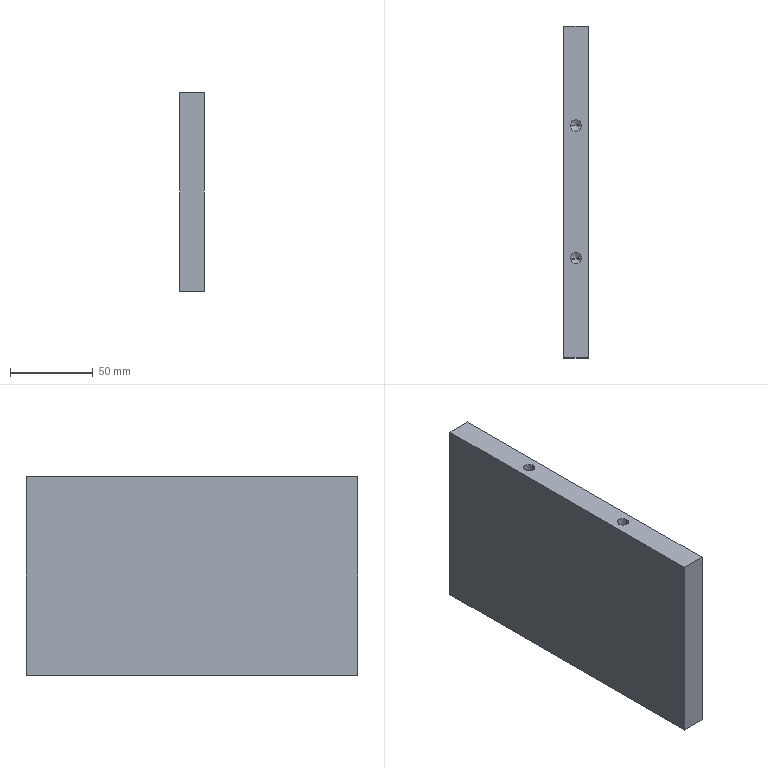Part | STEP file | 11-FGXW-07-0311 | 1 solid | 26 faces | box 15 x 200 x 120 mm | volume 356281 mm3 | cylinder 10 | cone 10 | plane 6 | commonest cylinder face diameters 6.8 x10
STEP:
#1=CARTESIAN_POINT('',(3.4,75.,19.8));
#2=VERTEX_POINT('',#1);
#3=CARTESIAN_POINT('',(-3.4,75.,19.8));
#4=VERTEX_POINT('',#3);
#5=CARTESIAN_POINT('',(0.,75.,19.8));
#6=DIRECTION('',(0.,0.,-1.));
#7=DIRECTION('',(-1.,0.,0.));
#8=AXIS2_PLACEMENT_3D('',#5,#6,#7);
#9=CIRCLE('',#8,3.4);
#10=EDGE_CURVE('',#2,#4,#9,.T.);
#11=ORIENTED_EDGE('',*,*,#10,.F.);
#12=CARTESIAN_POINT('',(3.4,75.,0.));
#13=VERTEX_POINT('',#12);
#14=CARTESIAN_POINT('',(3.4,75.,0.));
#15=DIRECTION('',(0.,0.,-1.));
#16=VECTOR('',#15,1000.);
#17=LINE('',#14,#16);
#18=EDGE_CURVE('',#2,#13,#17,.T.);
#19=ORIENTED_EDGE('',*,*,#18,.T.);
#20=CARTESIAN_POINT('',(-3.4,75.,0.));
#21=VERTEX_POINT('',#20);
#22=CARTESIAN_POINT('',(0.,75.,0.));
#23=DIRECTION('',(0.,0.,-1.));
#24=DIRECTION('',(-1.,0.,0.));
#25=AXIS2_PLACEMENT_3D('',#22,#23,#24);
#26=CIRCLE('',#25,3.4);
#27=EDGE_CURVE('',#13,#21,#26,.T.);
#28=ORIENTED_EDGE('',*,*,#27,.T.);
#29=CARTESIAN_POINT('',(-3.4,75.,0.));
#30=DIRECTION('',(0.,0.,-1.));
#31=VECTOR('',#30,1000.);
#32=LINE('',#29,#31);
#33=EDGE_CURVE('',#4,#21,#32,.T.);
#34=ORIENTED_EDGE('',*,*,#33,.F.);
#35=EDGE_LOOP('',(#11,#19,#28,#34));
#36=FACE_OUTER_BOUND('',#35,.T.);
#37=CARTESIAN_POINT('',(0.,75.,0.));
#38=DIRECTION('',(0.,0.,-1.));
#39=DIRECTION('',(-1.,0.,0.));
#40=AXIS2_PLACEMENT_3D('',#37,#38,#39);
#41=CYLINDRICAL_SURFACE('',#40,3.4);
#42=ADVANCED_FACE('',(#36),#41,.F.);
#43=CARTESIAN_POINT('',(0.,75.,21.843));
#44=VERTEX_POINT('',#43);
#45=CARTESIAN_POINT('',(-3.4,75.,19.8));
#46=DIRECTION('',(-0.8572,0.,-0.515));
#47=VECTOR('',#46,1000.);
#48=LINE('',#45,#47);
#49=EDGE_CURVE('',#44,#4,#48,.T.);
#50=ORIENTED_EDGE('',*,*,#49,.F.);
#51=CARTESIAN_POINT('',(3.4,75.,19.8));
#52=DIRECTION('',(0.8572,0.,-0.515));
#53=VECTOR('',#52,1000.);
#54=LINE('',#51,#53);
#55=EDGE_CURVE('',#44,#2,#54,.T.);
#56=ORIENTED_EDGE('',*,*,#55,.T.);
#57=ORIENTED_EDGE('',*,*,#10,.T.);
#58=EDGE_LOOP('',(#50,#56,#57));
#59=FACE_OUTER_BOUND('',#58,.T.);
#60=CARTESIAN_POINT('',(0.,75.,19.8));
#61=DIRECTION('',(0.,0.,-1.));
#62=DIRECTION('',(-1.,0.,0.));
#63=AXIS2_PLACEMENT_3D('',#60,#61,#62);
#64=CONICAL_SURFACE('',#63,3.4,1.03);
#65=ADVANCED_FACE('',(#59),#64,.F.);
#66=CARTESIAN_POINT('',(3.4,0.,19.8));
#67=VERTEX_POINT('',#66);
#68=CARTESIAN_POINT('',(-3.4,0.,19.8));
#69=VERTEX_POINT('',#68);
#70=CARTESIAN_POINT('',(0.,0.,19.8));
#71=DIRECTION('',(0.,0.,-1.));
#72=DIRECTION('',(-1.,0.,0.));
#73=AXIS2_PLACEMENT_3D('',#70,#71,#72);
#74=CIRCLE('',#73,3.4);
#75=EDGE_CURVE('',#67,#69,#74,.T.);
#76=ORIENTED_EDGE('',*,*,#75,.F.);
#77=CARTESIAN_POINT('',(3.4,0.,0.));
#78=VERTEX_POINT('',#77);
#79=CARTESIAN_POINT('',(3.4,0.,0.));
#80=DIRECTION('',(0.,0.,-1.));
#81=VECTOR('',#80,1000.);
#82=LINE('',#79,#81);
#83=EDGE_CURVE('',#67,#78,#82,.T.);
#84=ORIENTED_EDGE('',*,*,#83,.T.);
#85=CARTESIAN_POINT('',(-3.4,0.,0.));
#86=VERTEX_POINT('',#85);
#87=CARTESIAN_POINT('',(0.,0.,0.));
#88=DIRECTION('',(0.,0.,-1.));
#89=DIRECTION('',(-1.,0.,0.));
#90=AXIS2_PLACEMENT_3D('',#87,#88,#89);
#91=CIRCLE('',#90,3.4);
#92=EDGE_CURVE('',#78,#86,#91,.T.);
#93=ORIENTED_EDGE('',*,*,#92,.T.);
#94=CARTESIAN_POINT('',(-3.4,0.,0.));
#95=DIRECTION('',(0.,0.,-1.));
#96=VECTOR('',#95,1000.);
#97=LINE('',#94,#96);
#98=EDGE_CURVE('',#69,#86,#97,.T.);
#99=ORIENTED_EDGE('',*,*,#98,.F.);
#100=EDGE_LOOP('',(#76,#84,#93,#99));
#101=FACE_OUTER_BOUND('',#100,.T.);
#102=CARTESIAN_POINT('',(0.,0.,0.));
#103=DIRECTION('',(0.,0.,-1.));
#104=DIRECTION('',(-1.,0.,0.));
#105=AXIS2_PLACEMENT_3D('',#102,#103,#104);
#106=CYLINDRICAL_SURFACE('',#105,3.4);
#107=ADVANCED_FACE('',(#101),#106,.F.);
#108=CARTESIAN_POINT('',(0.,0.,21.843));
#109=VERTEX_POINT('',#108);
#110=CARTESIAN_POINT('',(-3.4,0.,19.8));
#111=DIRECTION('',(-0.8572,0.,-0.515));
#112=VECTOR('',#111,1000.);
#113=LINE('',#110,#112);
#114=EDGE_CURVE('',#109,#69,#113,.T.);
#115=ORIENTED_EDGE('',*,*,#114,.F.);
#116=CARTESIAN_POINT('',(3.4,0.,19.8));
#117=DIRECTION('',(0.8572,0.,-0.515));
#118=VECTOR('',#117,1000.);
#119=LINE('',#116,#118);
#120=EDGE_CURVE('',#109,#67,#119,.T.);
#121=ORIENTED_EDGE('',*,*,#120,.T.);
#122=ORIENTED_EDGE('',*,*,#75,.T.);
#123=EDGE_LOOP('',(#115,#121,#122));
#124=FACE_OUTER_BOUND('',#123,.T.);
#125=CARTESIAN_POINT('',(0.,0.,19.8));
#126=DIRECTION('',(0.,0.,-1.));
#127=DIRECTION('',(-1.,0.,0.));
#128=AXIS2_PLACEMENT_3D('',#125,#126,#127);
#129=CONICAL_SURFACE('',#128,3.4,1.03);
#130=ADVANCED_FACE('',(#124),#129,.F.);
#131=CARTESIAN_POINT('',(3.4,-75.,19.8));
#132=VERTEX_POINT('',#131);
#133=CARTESIAN_POINT('',(-3.4,-75.,19.8));
#134=VERTEX_POINT('',#133);
#135=CARTESIAN_POINT('',(0.,-75.,19.8));
#136=DIRECTION('',(0.,0.,-1.));
#137=DIRECTION('',(-1.,0.,0.));
#138=AXIS2_PLACEMENT_3D('',#135,#136,#137);
#139=CIRCLE('',#138,3.4);
#140=EDGE_CURVE('',#132,#134,#139,.T.);
#141=ORIENTED_EDGE('',*,*,#140,.F.);
#142=CARTESIAN_POINT('',(3.4,-75.,0.));
#143=VERTEX_POINT('',#142);
#144=CARTESIAN_POINT('',(3.4,-75.,0.));
#145=DIRECTION('',(0.,0.,-1.));
#146=VECTOR('',#145,1000.);
#147=LINE('',#144,#146);
#148=EDGE_CURVE('',#132,#143,#147,.T.);
#149=ORIENTED_EDGE('',*,*,#148,.T.);
#150=CARTESIAN_POINT('',(-3.4,-75.,0.));
#151=VERTEX_POINT('',#150);
#152=CARTESIAN_POINT('',(0.,-75.,0.));
#153=DIRECTION('',(0.,0.,-1.));
#154=DIRECTION('',(-1.,0.,0.));
#155=AXIS2_PLACEMENT_3D('',#152,#153,#154);
#156=CIRCLE('',#155,3.4);
#157=EDGE_CURVE('',#143,#151,#156,.T.);
#158=ORIENTED_EDGE('',*,*,#157,.T.);
#159=CARTESIAN_POINT('',(-3.4,-75.,0.));
#160=DIRECTION('',(0.,0.,-1.));
#161=VECTOR('',#160,1000.);
#162=LINE('',#159,#161);
#163=EDGE_CURVE('',#134,#151,#162,.T.);
#164=ORIENTED_EDGE('',*,*,#163,.F.);
#165=EDGE_LOOP('',(#141,#149,#158,#164));
#166=FACE_OUTER_BOUND('',#165,.T.);
#167=CARTESIAN_POINT('',(0.,-75.,0.));
#168=DIRECTION('',(0.,0.,-1.));
#169=DIRECTION('',(-1.,0.,0.));
#170=AXIS2_PLACEMENT_3D('',#167,#168,#169);
#171=CYLINDRICAL_SURFACE('',#170,3.4);
#172=ADVANCED_FACE('',(#166),#171,.F.);
#173=CARTESIAN_POINT('',(0.,-75.,21.843));
#174=VERTEX_POINT('',#173);
#175=CARTESIAN_POINT('',(-3.4,-75.,19.8));
#176=DIRECTION('',(-0.8572,0.,-0.515));
#177=VECTOR('',#176,1000.);
#178=LINE('',#175,#177);
#179=EDGE_CURVE('',#174,#134,#178,.T.);
#180=ORIENTED_EDGE('',*,*,#179,.F.);
#181=CARTESIAN_POINT('',(3.4,-75.,19.8));
#182=DIRECTION('',(0.8572,0.,-0.515));
#183=VECTOR('',#182,1000.);
#184=LINE('',#181,#183);
#185=EDGE_CURVE('',#174,#132,#184,.T.);
#186=ORIENTED_EDGE('',*,*,#185,.T.);
#187=ORIENTED_EDGE('',*,*,#140,.T.);
#188=EDGE_LOOP('',(#180,#186,#187));
#189=FACE_OUTER_BOUND('',#188,.T.);
#190=CARTESIAN_POINT('',(0.,-75.,19.8));
#191=DIRECTION('',(0.,0.,-1.));
#192=DIRECTION('',(-1.,0.,0.));
#193=AXIS2_PLACEMENT_3D('',#190,#191,#192);
#194=CONICAL_SURFACE('',#193,3.4,1.03);
#195=ADVANCED_FACE('',(#189),#194,.F.);
#196=CARTESIAN_POINT('',(-3.4,-40.,100.2));
#197=VERTEX_POINT('',#196);
#198=CARTESIAN_POINT('',(3.4,-40.,100.2));
#199=VERTEX_POINT('',#198);
#200=CARTESIAN_POINT('',(0.,-40.,100.2));
#201=DIRECTION('',(0.,0.,1.));
#202=DIRECTION('',(1.,0.,0.));
#203=AXIS2_PLACEMENT_3D('',#200,#201,#202);
#204=CIRCLE('',#203,3.4);
#205=EDGE_CURVE('',#197,#199,#204,.T.);
#206=ORIENTED_EDGE('',*,*,#205,.F.);
#207=CARTESIAN_POINT('',(-3.4,-40.,120.));
#208=VERTEX_POINT('',#207);
#209=CARTESIAN_POINT('',(-3.4,-40.,120.));
#210=DIRECTION('',(0.,0.,1.));
#211=VECTOR('',#210,1000.);
#212=LINE('',#209,#211);
#213=EDGE_CURVE('',#197,#208,#212,.T.);
#214=ORIENTED_EDGE('',*,*,#213,.T.);
#215=CARTESIAN_POINT('',(3.4,-40.,120.));
#216=VERTEX_POINT('',#215);
#217=CARTESIAN_POINT('',(0.,-40.,120.));
#218=DIRECTION('',(0.,0.,1.));
#219=DIRECTION('',(1.,0.,0.));
#220=AXIS2_PLACEMENT_3D('',#217,#218,#219);
#221=CIRCLE('',#220,3.4);
#222=EDGE_CURVE('',#208,#216,#221,.T.);
#223=ORIENTED_EDGE('',*,*,#222,.T.);
#224=CARTESIAN_POINT('',(3.4,-40.,120.));
#225=DIRECTION('',(0.,0.,1.));
#226=VECTOR('',#225,1000.);
#227=LINE('',#224,#226);
#228=EDGE_CURVE('',#199,#216,#227,.T.);
#229=ORIENTED_EDGE('',*,*,#228,.F.);
#230=EDGE_LOOP('',(#206,#214,#223,#229));
#231=FACE_OUTER_BOUND('',#230,.T.);
#232=CARTESIAN_POINT('',(0.,-40.,120.));
#233=DIRECTION('',(0.,0.,1.));
#234=DIRECTION('',(1.,0.,0.));
#235=AXIS2_PLACEMENT_3D('',#232,#233,#234);
#236=CYLINDRICAL_SURFACE('',#235,3.4);
#237=ADVANCED_FACE('',(#231),#236,.F.);
#238=CARTESIAN_POINT('',(0.,-40.,98.157));
#239=VERTEX_POINT('',#238);
#240=CARTESIAN_POINT('',(3.4,-40.,100.2));
#241=DIRECTION('',(0.8572,0.,0.515));
#242=VECTOR('',#241,1000.);
#243=LINE('',#240,#242);
#244=EDGE_CURVE('',#239,#199,#243,.T.);
#245=ORIENTED_EDGE('',*,*,#244,.F.);
#246=CARTESIAN_POINT('',(-3.4,-40.,100.2));
#247=DIRECTION('',(-0.8572,0.,0.515));
#248=VECTOR('',#247,1000.);
#249=LINE('',#246,#248);
#250=EDGE_CURVE('',#239,#197,#249,.T.);
#251=ORIENTED_EDGE('',*,*,#250,.T.);
#252=ORIENTED_EDGE('',*,*,#205,.T.);
#253=EDGE_LOOP('',(#245,#251,#252));
#254=FACE_OUTER_BOUND('',#253,.T.);
#255=CARTESIAN_POINT('',(0.,-40.,100.2));
#256=DIRECTION('',(0.,0.,1.));
#257=DIRECTION('',(1.,0.,0.));
#258=AXIS2_PLACEMENT_3D('',#255,#256,#257);
#259=CONICAL_SURFACE('',#258,3.4,1.03);
#260=ADVANCED_FACE('',(#254),#259,.F.);
#261=CARTESIAN_POINT('',(-3.4,40.,100.2));
#262=VERTEX_POINT('',#261);
#263=CARTESIAN_POINT('',(3.4,40.,100.2));
#264=VERTEX_POINT('',#263);
#265=CARTESIAN_POINT('',(0.,40.,100.2));
#266=DIRECTION('',(0.,0.,1.));
#267=DIRECTION('',(1.,0.,0.));
#268=AXIS2_PLACEMENT_3D('',#265,#266,#267);
#269=CIRCLE('',#268,3.4);
#270=EDGE_CURVE('',#262,#264,#269,.T.);
#271=ORIENTED_EDGE('',*,*,#270,.F.);
#272=CARTESIAN_POINT('',(-3.4,40.,120.));
#273=VERTEX_POINT('',#272);
#274=CARTESIAN_POINT('',(-3.4,40.,120.));
#275=DIRECTION('',(0.,0.,1.));
#276=VECTOR('',#275,1000.);
#277=LINE('',#274,#276);
#278=EDGE_CURVE('',#262,#273,#277,.T.);
#279=ORIENTED_EDGE('',*,*,#278,.T.);
#280=CARTESIAN_POINT('',(3.4,40.,120.));
#281=VERTEX_POINT('',#280);
#282=CARTESIAN_POINT('',(0.,40.,120.));
#283=DIRECTION('',(0.,0.,1.));
#284=DIRECTION('',(1.,0.,0.));
#285=AXIS2_PLACEMENT_3D('',#282,#283,#284);
#286=CIRCLE('',#285,3.4);
#287=EDGE_CURVE('',#273,#281,#286,.T.);
#288=ORIENTED_EDGE('',*,*,#287,.T.);
#289=CARTESIAN_POINT('',(3.4,40.,120.));
#290=DIRECTION('',(0.,0.,1.));
#291=VECTOR('',#290,1000.);
#292=LINE('',#289,#291);
#293=EDGE_CURVE('',#264,#281,#292,.T.);
#294=ORIENTED_EDGE('',*,*,#293,.F.);
#295=EDGE_LOOP('',(#271,#279,#288,#294));
#296=FACE_OUTER_BOUND('',#295,.T.);
#297=CARTESIAN_POINT('',(0.,40.,120.));
#298=DIRECTION('',(0.,0.,1.));
#299=DIRECTION('',(1.,0.,0.));
#300=AXIS2_PLACEMENT_3D('',#297,#298,#299);
#301=CYLINDRICAL_SURFACE('',#300,3.4);
#302=ADVANCED_FACE('',(#296),#301,.F.);
#303=CARTESIAN_POINT('',(0.,40.,98.157));
#304=VERTEX_POINT('',#303);
#305=CARTESIAN_POINT('',(3.4,40.,100.2));
#306=DIRECTION('',(0.8572,0.,0.515));
#307=VECTOR('',#306,1000.);
#308=LINE('',#305,#307);
#309=EDGE_CURVE('',#304,#264,#308,.T.);
#310=ORIENTED_EDGE('',*,*,#309,.F.);
#311=CARTESIAN_POINT('',(-3.4,40.,100.2));
#312=DIRECTION('',(-0.8572,0.,0.515));
#313=VECTOR('',#312,1000.);
#314=LINE('',#311,#313);
#315=EDGE_CURVE('',#304,#262,#314,.T.);
#316=ORIENTED_EDGE('',*,*,#315,.T.);
#317=ORIENTED_EDGE('',*,*,#270,.T.);
#318=EDGE_LOOP('',(#310,#316,#317));
#319=FACE_OUTER_BOUND('',#318,.T.);
#320=CARTESIAN_POINT('',(0.,40.,100.2));
#321=DIRECTION('',(0.,0.,1.));
#322=DIRECTION('',(1.,0.,0.));
#323=AXIS2_PLACEMENT_3D('',#320,#321,#322);
#324=CONICAL_SURFACE('',#323,3.4,1.03);
#325=ADVANCED_FACE('',(#319),#324,.F.);
#326=CARTESIAN_POINT('',(7.5,-100.,0.));
#327=VERTEX_POINT('',#326);
#328=CARTESIAN_POINT('',(7.5,100.,0.));
#329=VERTEX_POINT('',#328);
#330=CARTESIAN_POINT('',(7.5,-100.,0.));
#331=DIRECTION('',(0.,1.,0.));
#332=VECTOR('',#331,1000.);
#333=LINE('',#330,#332);
#334=EDGE_CURVE('',#327,#329,#333,.T.);
#335=ORIENTED_EDGE('',*,*,#334,.T.);
#336=CARTESIAN_POINT('',(7.5,100.,120.));
#337=VERTEX_POINT('',#336);
#338=CARTESIAN_POINT('',(7.5,100.,120.));
#339=DIRECTION('',(0.,0.,-1.));
#340=VECTOR('',#339,1000.);
#341=LINE('',#338,#340);
#342=EDGE_CURVE('',#337,#329,#341,.T.);
#343=ORIENTED_EDGE('',*,*,#342,.F.);
#344=CARTESIAN_POINT('',(7.5,-100.,120.));
#345=VERTEX_POINT('',#344);
#346=CARTESIAN_POINT('',(7.5,-100.,120.));
#347=DIRECTION('',(0.,1.,0.));
#348=VECTOR('',#347,1000.);
#349=LINE('',#346,#348);
#350=EDGE_CURVE('',#345,#337,#349,.T.);
#351=ORIENTED_EDGE('',*,*,#350,.F.);
#352=CARTESIAN_POINT('',(7.5,-100.,120.));
#353=DIRECTION('',(0.,0.,-1.));
#354=VECTOR('',#353,1000.);
#355=LINE('',#352,#354);
#356=EDGE_CURVE('',#345,#327,#355,.T.);
#357=ORIENTED_EDGE('',*,*,#356,.T.);
#358=EDGE_LOOP('',(#335,#343,#351,#357));
#359=FACE_OUTER_BOUND('',#358,.T.);
#360=CARTESIAN_POINT('',(7.5,-100.,120.));
#361=DIRECTION('',(-1.,0.,0.));
#362=DIRECTION('',(0.,0.,1.));
#363=AXIS2_PLACEMENT_3D('',#360,#361,#362);
#364=PLANE('',#363);
#365=ADVANCED_FACE('',(#359),#364,.F.);
#366=CARTESIAN_POINT('',(-7.5,100.,0.));
#367=VERTEX_POINT('',#366);
#368=CARTESIAN_POINT('',(-7.5,100.,0.));
#369=DIRECTION('',(-1.,0.,0.));
#370=VECTOR('',#369,1000.);
#371=LINE('',#368,#370);
#372=EDGE_CURVE('',#329,#367,#371,.T.);
#373=ORIENTED_EDGE('',*,*,#372,.T.);
#374=CARTESIAN_POINT('',(-7.5,100.,120.));
#375=VERTEX_POINT('',#374);
#376=CARTESIAN_POINT('',(-7.5,100.,120.));
#377=DIRECTION('',(0.,0.,-1.));
#378=VECTOR('',#377,1000.);
#379=LINE('',#376,#378);
#380=EDGE_CURVE('',#375,#367,#379,.T.);
#381=ORIENTED_EDGE('',*,*,#380,.F.);
#382=CARTESIAN_POINT('',(-7.5,100.,120.));
#383=DIRECTION('',(-1.,0.,0.));
#384=VECTOR('',#383,1000.);
#385=LINE('',#382,#384);
#386=EDGE_CURVE('',#337,#375,#385,.T.);
#387=ORIENTED_EDGE('',*,*,#386,.F.);
#388=ORIENTED_EDGE('',*,*,#342,.T.);
#389=EDGE_LOOP('',(#373,#381,#387,#388));
#390=FACE_OUTER_BOUND('',#389,.T.);
#391=CARTESIAN_POINT('',(-7.5,100.,120.));
#392=DIRECTION('',(0.,-1.,0.));
#393=DIRECTION('',(0.,0.,-1.));
#394=AXIS2_PLACEMENT_3D('',#391,#392,#393);
#395=PLANE('',#394);
#396=ADVANCED_FACE('',(#390),#395,.F.);
#397=CARTESIAN_POINT('',(-7.5,-100.,0.));
#398=VERTEX_POINT('',#397);
#399=CARTESIAN_POINT('',(-7.5,-100.,0.));
#400=DIRECTION('',(0.,-1.,0.));
#401=VECTOR('',#400,1000.);
#402=LINE('',#399,#401);
#403=EDGE_CURVE('',#367,#398,#402,.T.);
#404=ORIENTED_EDGE('',*,*,#403,.T.);
#405=CARTESIAN_POINT('',(-7.5,-100.,120.));
#406=VERTEX_POINT('',#405);
#407=CARTESIAN_POINT('',(-7.5,-100.,120.));
#408=DIRECTION('',(0.,0.,-1.));
#409=VECTOR('',#408,1000.);
#410=LINE('',#407,#409);
#411=EDGE_CURVE('',#406,#398,#410,.T.);
#412=ORIENTED_EDGE('',*,*,#411,.F.);
#413=CARTESIAN_POINT('',(-7.5,-100.,120.));
#414=DIRECTION('',(0.,-1.,0.));
#415=VECTOR('',#414,1000.);
#416=LINE('',#413,#415);
#417=EDGE_CURVE('',#375,#406,#416,.T.);
#418=ORIENTED_EDGE('',*,*,#417,.F.);
#419=ORIENTED_EDGE('',*,*,#380,.T.);
#420=EDGE_LOOP('',(#404,#412,#418,#419));
#421=FACE_OUTER_BOUND('',#420,.T.);
#422=CARTESIAN_POINT('',(-7.5,-100.,120.));
#423=DIRECTION('',(1.,0.,0.));
#424=DIRECTION('',(0.,0.,-1.));
#425=AXIS2_PLACEMENT_3D('',#422,#423,#424);
#426=PLANE('',#425);
#427=ADVANCED_FACE('',(#421),#426,.F.);
#428=CARTESIAN_POINT('',(-7.5,-100.,0.));
#429=DIRECTION('',(1.,0.,0.));
#430=VECTOR('',#429,1000.);
#431=LINE('',#428,#430);
#432=EDGE_CURVE('',#398,#327,#431,.T.);
#433=ORIENTED_EDGE('',*,*,#432,.T.);
#434=ORIENTED_EDGE('',*,*,#356,.F.);
#435=CARTESIAN_POINT('',(-7.5,-100.,120.));
#436=DIRECTION('',(1.,0.,0.));
#437=VECTOR('',#436,1000.);
#438=LINE('',#435,#437);
#439=EDGE_CURVE('',#406,#345,#438,.T.);
#440=ORIENTED_EDGE('',*,*,#439,.F.);
#441=ORIENTED_EDGE('',*,*,#411,.T.);
#442=EDGE_LOOP('',(#433,#434,#440,#441));
#443=FACE_OUTER_BOUND('',#442,.T.);
#444=CARTESIAN_POINT('',(-7.5,-100.,120.));
#445=DIRECTION('',(0.,1.,0.));
#446=DIRECTION('',(0.,0.,1.));
#447=AXIS2_PLACEMENT_3D('',#444,#445,#446);
#448=PLANE('',#447);
#449=ADVANCED_FACE('',(#443),#448,.F.);
#450=CARTESIAN_POINT('',(0.,-40.,120.));
#451=DIRECTION('',(0.,0.,1.));
#452=DIRECTION('',(1.,0.,0.));
#453=AXIS2_PLACEMENT_3D('',#450,#451,#452);
#454=CIRCLE('',#453,3.4);
#455=EDGE_CURVE('',#216,#208,#454,.T.);
#456=ORIENTED_EDGE('',*,*,#455,.F.);
#457=ORIENTED_EDGE('',*,*,#222,.F.);
#458=EDGE_LOOP('',(#456,#457));
#459=FACE_BOUND('',#458,.T.);
#460=CARTESIAN_POINT('',(0.,40.,120.));
#461=DIRECTION('',(0.,0.,1.));
#462=DIRECTION('',(1.,0.,0.));
#463=AXIS2_PLACEMENT_3D('',#460,#461,#462);
#464=CIRCLE('',#463,3.4);
#465=EDGE_CURVE('',#281,#273,#464,.T.);
#466=ORIENTED_EDGE('',*,*,#465,.F.);
#467=ORIENTED_EDGE('',*,*,#287,.F.);
#468=EDGE_LOOP('',(#466,#467));
#469=FACE_BOUND('',#468,.T.);
#470=ORIENTED_EDGE('',*,*,#350,.T.);
#471=ORIENTED_EDGE('',*,*,#386,.T.);
#472=ORIENTED_EDGE('',*,*,#417,.T.);
#473=ORIENTED_EDGE('',*,*,#439,.T.);
#474=EDGE_LOOP('',(#470,#471,#472,#473));
#475=FACE_OUTER_BOUND('',#474,.T.);
#476=CARTESIAN_POINT('',(0.,0.,120.));
#477=DIRECTION('',(0.,0.,-1.));
#478=DIRECTION('',(-1.,0.,0.));
#479=AXIS2_PLACEMENT_3D('',#476,#477,#478);
#480=PLANE('',#479);
#481=ADVANCED_FACE('',(#459,#469,#475),#480,.F.);
#482=CARTESIAN_POINT('',(0.,75.,0.));
#483=DIRECTION('',(0.,0.,-1.));
#484=DIRECTION('',(-1.,0.,0.));
#485=AXIS2_PLACEMENT_3D('',#482,#483,#484);
#486=CIRCLE('',#485,3.4);
#487=EDGE_CURVE('',#21,#13,#486,.T.);
#488=ORIENTED_EDGE('',*,*,#487,.F.);
#489=ORIENTED_EDGE('',*,*,#27,.F.);
#490=EDGE_LOOP('',(#488,#489));
#491=FACE_BOUND('',#490,.T.);
#492=CARTESIAN_POINT('',(0.,0.,0.));
#493=DIRECTION('',(0.,0.,-1.));
#494=DIRECTION('',(-1.,0.,0.));
#495=AXIS2_PLACEMENT_3D('',#492,#493,#494);
#496=CIRCLE('',#495,3.4);
#497=EDGE_CURVE('',#86,#78,#496,.T.);
#498=ORIENTED_EDGE('',*,*,#497,.F.);
#499=ORIENTED_EDGE('',*,*,#92,.F.);
#500=EDGE_LOOP('',(#498,#499));
#501=FACE_BOUND('',#500,.T.);
#502=CARTESIAN_POINT('',(0.,-75.,0.));
#503=DIRECTION('',(0.,0.,-1.));
#504=DIRECTION('',(-1.,0.,0.));
#505=AXIS2_PLACEMENT_3D('',#502,#503,#504);
#506=CIRCLE('',#505,3.4);
#507=EDGE_CURVE('',#151,#143,#506,.T.);
#508=ORIENTED_EDGE('',*,*,#507,.F.);
#509=ORIENTED_EDGE('',*,*,#157,.F.);
#510=EDGE_LOOP('',(#508,#509));
#511=FACE_BOUND('',#510,.T.);
#512=ORIENTED_EDGE('',*,*,#334,.F.);
#513=ORIENTED_EDGE('',*,*,#432,.F.);
#514=ORIENTED_EDGE('',*,*,#403,.F.);
#515=ORIENTED_EDGE('',*,*,#372,.F.);
#516=EDGE_LOOP('',(#512,#513,#514,#515));
#517=FACE_OUTER_BOUND('',#516,.T.);
#518=CARTESIAN_POINT('',(0.,0.,0.));
#519=DIRECTION('',(0.,0.,-1.));
#520=DIRECTION('',(-1.,0.,0.));
#521=AXIS2_PLACEMENT_3D('',#518,#519,#520);
#522=PLANE('',#521);
#523=ADVANCED_FACE('',(#491,#501,#511,#517),#522,.T.);
#524=ORIENTED_EDGE('',*,*,#315,.F.);
#525=ORIENTED_EDGE('',*,*,#309,.T.);
#526=CARTESIAN_POINT('',(0.,40.,100.2));
#527=DIRECTION('',(0.,0.,1.));
#528=DIRECTION('',(1.,0.,0.));
#529=AXIS2_PLACEMENT_3D('',#526,#527,#528);
#530=CIRCLE('',#529,3.4);
#531=EDGE_CURVE('',#264,#262,#530,.T.);
#532=ORIENTED_EDGE('',*,*,#531,.T.);
#533=EDGE_LOOP('',(#524,#525,#532));
#534=FACE_OUTER_BOUND('',#533,.T.);
#535=CARTESIAN_POINT('',(0.,40.,100.2));
#536=DIRECTION('',(0.,0.,1.));
#537=DIRECTION('',(1.,0.,0.));
#538=AXIS2_PLACEMENT_3D('',#535,#536,#537);
#539=CONICAL_SURFACE('',#538,3.4,1.03);
#540=ADVANCED_FACE('',(#534),#539,.F.);
#541=ORIENTED_EDGE('',*,*,#278,.F.);
#542=ORIENTED_EDGE('',*,*,#531,.F.);
#543=ORIENTED_EDGE('',*,*,#293,.T.);
#544=ORIENTED_EDGE('',*,*,#465,.T.);
#545=EDGE_LOOP('',(#541,#542,#543,#544));
#546=FACE_OUTER_BOUND('',#545,.T.);
#547=CARTESIAN_POINT('',(0.,40.,120.));
#548=DIRECTION('',(0.,0.,1.));
#549=DIRECTION('',(1.,0.,0.));
#550=AXIS2_PLACEMENT_3D('',#547,#548,#549);
#551=CYLINDRICAL_SURFACE('',#550,3.4);
#552=ADVANCED_FACE('',(#546),#551,.F.);
#553=ORIENTED_EDGE('',*,*,#250,.F.);
#554=ORIENTED_EDGE('',*,*,#244,.T.);
#555=CARTESIAN_POINT('',(0.,-40.,100.2));
#556=DIRECTION('',(0.,0.,1.));
#557=DIRECTION('',(1.,0.,0.));
#558=AXIS2_PLACEMENT_3D('',#555,#556,#557);
#559=CIRCLE('',#558,3.4);
#560=EDGE_CURVE('',#199,#197,#559,.T.);
#561=ORIENTED_EDGE('',*,*,#560,.T.);
#562=EDGE_LOOP('',(#553,#554,#561));
#563=FACE_OUTER_BOUND('',#562,.T.);
#564=CARTESIAN_POINT('',(0.,-40.,100.2));
#565=DIRECTION('',(0.,0.,1.));
#566=DIRECTION('',(1.,0.,0.));
#567=AXIS2_PLACEMENT_3D('',#564,#565,#566);
#568=CONICAL_SURFACE('',#567,3.4,1.03);
#569=ADVANCED_FACE('',(#563),#568,.F.);
#570=ORIENTED_EDGE('',*,*,#213,.F.);
#571=ORIENTED_EDGE('',*,*,#560,.F.);
#572=ORIENTED_EDGE('',*,*,#228,.T.);
#573=ORIENTED_EDGE('',*,*,#455,.T.);
#574=EDGE_LOOP('',(#570,#571,#572,#573));
#575=FACE_OUTER_BOUND('',#574,.T.);
#576=CARTESIAN_POINT('',(0.,-40.,120.));
#577=DIRECTION('',(0.,0.,1.));
#578=DIRECTION('',(1.,0.,0.));
#579=AXIS2_PLACEMENT_3D('',#576,#577,#578);
#580=CYLINDRICAL_SURFACE('',#579,3.4);
#581=ADVANCED_FACE('',(#575),#580,.F.);
#582=ORIENTED_EDGE('',*,*,#185,.F.);
#583=ORIENTED_EDGE('',*,*,#179,.T.);
#584=CARTESIAN_POINT('',(0.,-75.,19.8));
#585=DIRECTION('',(0.,0.,-1.));
#586=DIRECTION('',(-1.,0.,0.));
#587=AXIS2_PLACEMENT_3D('',#584,#585,#586);
#588=CIRCLE('',#587,3.4);
#589=EDGE_CURVE('',#134,#132,#588,.T.);
#590=ORIENTED_EDGE('',*,*,#589,.T.);
#591=EDGE_LOOP('',(#582,#583,#590));
#592=FACE_OUTER_BOUND('',#591,.T.);
#593=CARTESIAN_POINT('',(0.,-75.,19.8));
#594=DIRECTION('',(0.,0.,-1.));
#595=DIRECTION('',(-1.,0.,0.));
#596=AXIS2_PLACEMENT_3D('',#593,#594,#595);
#597=CONICAL_SURFACE('',#596,3.4,1.03);
#598=ADVANCED_FACE('',(#592),#597,.F.);
#599=ORIENTED_EDGE('',*,*,#148,.F.);
#600=ORIENTED_EDGE('',*,*,#589,.F.);
#601=ORIENTED_EDGE('',*,*,#163,.T.);
#602=ORIENTED_EDGE('',*,*,#507,.T.);
#603=EDGE_LOOP('',(#599,#600,#601,#602));
#604=FACE_OUTER_BOUND('',#603,.T.);
#605=CARTESIAN_POINT('',(0.,-75.,0.));
#606=DIRECTION('',(0.,0.,-1.));
#607=DIRECTION('',(-1.,0.,0.));
#608=AXIS2_PLACEMENT_3D('',#605,#606,#607);
#609=CYLINDRICAL_SURFACE('',#608,3.4);
#610=ADVANCED_FACE('',(#604),#609,.F.);
#611=ORIENTED_EDGE('',*,*,#120,.F.);
#612=ORIENTED_EDGE('',*,*,#114,.T.);
#613=CARTESIAN_POINT('',(0.,0.,19.8));
#614=DIRECTION('',(0.,0.,-1.));
#615=DIRECTION('',(-1.,0.,0.));
#616=AXIS2_PLACEMENT_3D('',#613,#614,#615);
#617=CIRCLE('',#616,3.4);
#618=EDGE_CURVE('',#69,#67,#617,.T.);
#619=ORIENTED_EDGE('',*,*,#618,.T.);
#620=EDGE_LOOP('',(#611,#612,#619));
#621=FACE_OUTER_BOUND('',#620,.T.);
#622=CARTESIAN_POINT('',(0.,0.,19.8));
#623=DIRECTION('',(0.,0.,-1.));
#624=DIRECTION('',(-1.,0.,0.));
#625=AXIS2_PLACEMENT_3D('',#622,#623,#624);
#626=CONICAL_SURFACE('',#625,3.4,1.03);
#627=ADVANCED_FACE('',(#621),#626,.F.);
#628=ORIENTED_EDGE('',*,*,#83,.F.);
#629=ORIENTED_EDGE('',*,*,#618,.F.);
#630=ORIENTED_EDGE('',*,*,#98,.T.);
#631=ORIENTED_EDGE('',*,*,#497,.T.);
#632=EDGE_LOOP('',(#628,#629,#630,#631));
#633=FACE_OUTER_BOUND('',#632,.T.);
#634=CARTESIAN_POINT('',(0.,0.,0.));
#635=DIRECTION('',(0.,0.,-1.));
#636=DIRECTION('',(-1.,0.,0.));
#637=AXIS2_PLACEMENT_3D('',#634,#635,#636);
#638=CYLINDRICAL_SURFACE('',#637,3.4);
#639=ADVANCED_FACE('',(#633),#638,.F.);
#640=ORIENTED_EDGE('',*,*,#55,.F.);
#641=ORIENTED_EDGE('',*,*,#49,.T.);
#642=CARTESIAN_POINT('',(0.,75.,19.8));
#643=DIRECTION('',(0.,0.,-1.));
#644=DIRECTION('',(-1.,0.,0.));
#645=AXIS2_PLACEMENT_3D('',#642,#643,#644);
#646=CIRCLE('',#645,3.4);
#647=EDGE_CURVE('',#4,#2,#646,.T.);
#648=ORIENTED_EDGE('',*,*,#647,.T.);
#649=EDGE_LOOP('',(#640,#641,#648));
#650=FACE_OUTER_BOUND('',#649,.T.);
#651=CARTESIAN_POINT('',(0.,75.,19.8));
#652=DIRECTION('',(0.,0.,-1.));
#653=DIRECTION('',(-1.,0.,0.));
#654=AXIS2_PLACEMENT_3D('',#651,#652,#653);
#655=CONICAL_SURFACE('',#654,3.4,1.03);
#656=ADVANCED_FACE('',(#650),#655,.F.);
#657=ORIENTED_EDGE('',*,*,#18,.F.);
#658=ORIENTED_EDGE('',*,*,#647,.F.);
#659=ORIENTED_EDGE('',*,*,#33,.T.);
#660=ORIENTED_EDGE('',*,*,#487,.T.);
#661=EDGE_LOOP('',(#657,#658,#659,#660));
#662=FACE_OUTER_BOUND('',#661,.T.);
#663=CARTESIAN_POINT('',(0.,75.,0.));
#664=DIRECTION('',(0.,0.,-1.));
#665=DIRECTION('',(-1.,0.,0.));
#666=AXIS2_PLACEMENT_3D('',#663,#664,#665);
#667=CYLINDRICAL_SURFACE('',#666,3.4);
#668=ADVANCED_FACE('',(#662),#667,.F.);
#669=CLOSED_SHELL('',(#42,#65,#107,#130,#172,#195,#237,#260,#302,#325,#365,#396,#427,#449,#481,#523,#540,#552,#569,#581,#598,#610,#627,#639,#656,#668));
#670=MANIFOLD_SOLID_BREP('',#669);
#671=CARTESIAN_POINT('',(0.,0.,0.));
#672=DIRECTION('',(0.,0.,1.));
#673=DIRECTION('',(1.,0.,0.));
#674=AXIS2_PLACEMENT_3D('',#671,#672,#673);
#675=(LENGTH_UNIT()NAMED_UNIT(*)SI_UNIT(.MILLI.,.METRE.));
#676=UNCERTAINTY_MEASURE_WITH_UNIT(LENGTH_MEASURE(0.00001),#675,'','');
#677=(NAMED_UNIT(*)PLANE_ANGLE_UNIT()SI_UNIT($,.RADIAN.));
#678=(NAMED_UNIT(*)SI_UNIT($,.STERADIAN.)SOLID_ANGLE_UNIT());
#679=(GEOMETRIC_REPRESENTATION_CONTEXT(3)GLOBAL_UNCERTAINTY_ASSIGNED_CONTEXT((#676))GLOBAL_UNIT_ASSIGNED_CONTEXT((#675,#677,#678))REPRESENTATION_CONTEXT('',''));
#680=ADVANCED_BREP_SHAPE_REPRESENTATION('',(#670,#674),#679);